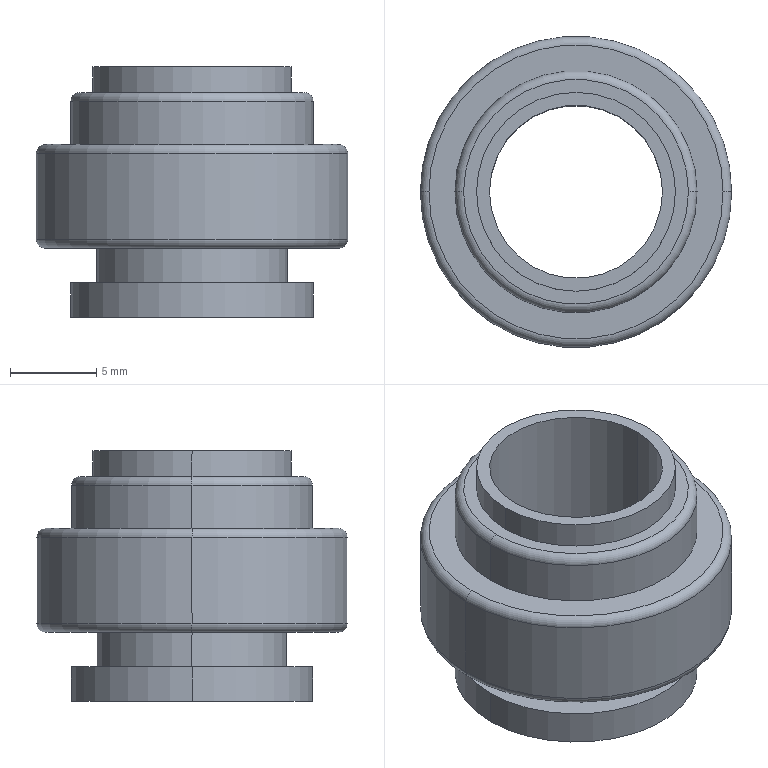Part | SolidWorks | features BaseBody 1 | 1 solid | 24 faces | box 18 x 18 x 14.5 mm | volume 1495 mm3 | cylinder 12 | plane 6 | torus 6 | commonest cylinder face diameters 14 x4 10 x2 11 x2 11.5 x2 18 x2
STEP:
#1=CARTESIAN_POINT('',(5.75,-5.,5.75));
#2=VERTEX_POINT('',#1);
#3=CARTESIAN_POINT('',(-5.75,-5.,5.75));
#4=VERTEX_POINT('',#3);
#5=CARTESIAN_POINT('',(0.,-5.,5.75));
#6=DIRECTION('',(0.,0.,1.));
#7=DIRECTION('',(1.,0.,0.));
#8=AXIS2_PLACEMENT_3D('',#5,#6,#7);
#9=CIRCLE('',#8,5.75);
#10=EDGE_CURVE('',#2,#4,#9,.T.);
#11=ORIENTED_EDGE('',*,*,#10,.F.);
#12=CARTESIAN_POINT('',(0.,-5.,5.75));
#13=DIRECTION('',(0.,0.,1.));
#14=DIRECTION('',(1.,0.,0.));
#15=AXIS2_PLACEMENT_3D('',#12,#13,#14);
#16=CIRCLE('',#15,5.75);
#17=EDGE_CURVE('',#4,#2,#16,.T.);
#18=ORIENTED_EDGE('',*,*,#17,.F.);
#19=EDGE_LOOP('',(#11,#18));
#20=FACE_BOUND('',#19,.T.);
#21=CARTESIAN_POINT('',(6.5,-5.,5.75));
#22=VERTEX_POINT('',#21);
#23=CARTESIAN_POINT('',(-6.5,-5.,5.75));
#24=VERTEX_POINT('',#23);
#25=CARTESIAN_POINT('',(0.,-5.,5.75));
#26=DIRECTION('',(0.,0.,1.));
#27=DIRECTION('',(1.,0.,0.));
#28=AXIS2_PLACEMENT_3D('',#25,#26,#27);
#29=CIRCLE('',#28,6.5);
#30=EDGE_CURVE('',#22,#24,#29,.T.);
#31=ORIENTED_EDGE('',*,*,#30,.T.);
#32=CARTESIAN_POINT('',(0.,-5.,5.75));
#33=DIRECTION('',(0.,0.,1.));
#34=DIRECTION('',(1.,0.,0.));
#35=AXIS2_PLACEMENT_3D('',#32,#33,#34);
#36=CIRCLE('',#35,6.5);
#37=EDGE_CURVE('',#24,#22,#36,.T.);
#38=ORIENTED_EDGE('',*,*,#37,.T.);
#39=EDGE_LOOP('',(#31,#38));
#40=FACE_OUTER_BOUND('',#39,.T.);
#41=CARTESIAN_POINT('',(0.,1.5,5.75));
#42=DIRECTION('',(0.,0.,-1.));
#43=DIRECTION('',(0.,-1.,0.));
#44=AXIS2_PLACEMENT_3D('',#41,#42,#43);
#45=PLANE('',#44);
#46=ADVANCED_FACE('',(#20,#40),#45,.F.);
#47=CARTESIAN_POINT('',(-5.75,-5.,7.25));
#48=VERTEX_POINT('',#47);
#49=CARTESIAN_POINT('',(-5.75,-5.,7.25));
#50=DIRECTION('',(0.,0.,1.));
#51=VECTOR('',#50,1000.);
#52=LINE('',#49,#51);
#53=EDGE_CURVE('',#4,#48,#52,.T.);
#54=ORIENTED_EDGE('',*,*,#53,.F.);
#55=ORIENTED_EDGE('',*,*,#17,.T.);
#56=CARTESIAN_POINT('',(5.75,-5.,7.25));
#57=VERTEX_POINT('',#56);
#58=CARTESIAN_POINT('',(5.75,-5.,7.25));
#59=DIRECTION('',(0.,0.,1.));
#60=VECTOR('',#59,1000.);
#61=LINE('',#58,#60);
#62=EDGE_CURVE('',#2,#57,#61,.T.);
#63=ORIENTED_EDGE('',*,*,#62,.T.);
#64=CARTESIAN_POINT('',(0.,-5.,7.25));
#65=DIRECTION('',(0.,0.,1.));
#66=DIRECTION('',(1.,0.,0.));
#67=AXIS2_PLACEMENT_3D('',#64,#65,#66);
#68=CIRCLE('',#67,5.75);
#69=EDGE_CURVE('',#48,#57,#68,.T.);
#70=ORIENTED_EDGE('',*,*,#69,.F.);
#71=EDGE_LOOP('',(#54,#55,#63,#70));
#72=FACE_OUTER_BOUND('',#71,.T.);
#73=CARTESIAN_POINT('',(0.,-5.,7.25));
#74=DIRECTION('',(0.,0.,1.));
#75=DIRECTION('',(1.,0.,0.));
#76=AXIS2_PLACEMENT_3D('',#73,#74,#75);
#77=CYLINDRICAL_SURFACE('',#76,5.75);
#78=ADVANCED_FACE('',(#72),#77,.T.);
#79=CARTESIAN_POINT('',(5.,-5.,7.25));
#80=VERTEX_POINT('',#79);
#81=CARTESIAN_POINT('',(-5.,-5.,7.25));
#82=VERTEX_POINT('',#81);
#83=CARTESIAN_POINT('',(0.,-5.,7.25));
#84=DIRECTION('',(0.,0.,1.));
#85=DIRECTION('',(1.,0.,0.));
#86=AXIS2_PLACEMENT_3D('',#83,#84,#85);
#87=CIRCLE('',#86,5.);
#88=EDGE_CURVE('',#80,#82,#87,.T.);
#89=ORIENTED_EDGE('',*,*,#88,.F.);
#90=CARTESIAN_POINT('',(0.,-5.,7.25));
#91=DIRECTION('',(0.,0.,1.));
#92=DIRECTION('',(1.,0.,0.));
#93=AXIS2_PLACEMENT_3D('',#90,#91,#92);
#94=CIRCLE('',#93,5.);
#95=EDGE_CURVE('',#82,#80,#94,.T.);
#96=ORIENTED_EDGE('',*,*,#95,.F.);
#97=EDGE_LOOP('',(#89,#96));
#98=FACE_BOUND('',#97,.T.);
#99=CARTESIAN_POINT('',(0.,-5.,7.25));
#100=DIRECTION('',(0.,0.,1.));
#101=DIRECTION('',(1.,0.,0.));
#102=AXIS2_PLACEMENT_3D('',#99,#100,#101);
#103=CIRCLE('',#102,5.75);
#104=EDGE_CURVE('',#57,#48,#103,.T.);
#105=ORIENTED_EDGE('',*,*,#104,.T.);
#106=ORIENTED_EDGE('',*,*,#69,.T.);
#107=EDGE_LOOP('',(#105,#106));
#108=FACE_OUTER_BOUND('',#107,.T.);
#109=CARTESIAN_POINT('',(0.,0.75,7.25));
#110=DIRECTION('',(0.,0.,-1.));
#111=DIRECTION('',(0.,-1.,0.));
#112=AXIS2_PLACEMENT_3D('',#109,#110,#111);
#113=PLANE('',#112);
#114=ADVANCED_FACE('',(#98,#108),#113,.F.);
#115=CARTESIAN_POINT('',(-5.,-5.,-7.25));
#116=VERTEX_POINT('',#115);
#117=CARTESIAN_POINT('',(-5.,-5.,7.25));
#118=DIRECTION('',(0.,0.,1.));
#119=VECTOR('',#118,1000.);
#120=LINE('',#117,#119);
#121=EDGE_CURVE('',#116,#82,#120,.T.);
#122=ORIENTED_EDGE('',*,*,#121,.F.);
#123=CARTESIAN_POINT('',(5.,-5.,-7.25));
#124=VERTEX_POINT('',#123);
#125=CARTESIAN_POINT('',(0.,-5.,-7.25));
#126=DIRECTION('',(0.,0.,1.));
#127=DIRECTION('',(1.,0.,0.));
#128=AXIS2_PLACEMENT_3D('',#125,#126,#127);
#129=CIRCLE('',#128,5.);
#130=EDGE_CURVE('',#124,#116,#129,.T.);
#131=ORIENTED_EDGE('',*,*,#130,.F.);
#132=CARTESIAN_POINT('',(5.,-5.,7.25));
#133=DIRECTION('',(0.,0.,1.));
#134=VECTOR('',#133,1000.);
#135=LINE('',#132,#134);
#136=EDGE_CURVE('',#124,#80,#135,.T.);
#137=ORIENTED_EDGE('',*,*,#136,.T.);
#138=ORIENTED_EDGE('',*,*,#88,.T.);
#139=EDGE_LOOP('',(#122,#131,#137,#138));
#140=FACE_OUTER_BOUND('',#139,.T.);
#141=CARTESIAN_POINT('',(0.,-5.,7.25));
#142=DIRECTION('',(0.,0.,1.));
#143=DIRECTION('',(1.,0.,0.));
#144=AXIS2_PLACEMENT_3D('',#141,#142,#143);
#145=CYLINDRICAL_SURFACE('',#144,5.);
#146=ADVANCED_FACE('',(#140),#145,.F.);
#147=ORIENTED_EDGE('',*,*,#130,.T.);
#148=CARTESIAN_POINT('',(0.,-5.,-7.25));
#149=DIRECTION('',(0.,0.,1.));
#150=DIRECTION('',(1.,0.,0.));
#151=AXIS2_PLACEMENT_3D('',#148,#149,#150);
#152=CIRCLE('',#151,5.);
#153=EDGE_CURVE('',#116,#124,#152,.T.);
#154=ORIENTED_EDGE('',*,*,#153,.T.);
#155=EDGE_LOOP('',(#147,#154));
#156=FACE_BOUND('',#155,.T.);
#157=CARTESIAN_POINT('',(7.,-5.,-7.25));
#158=VERTEX_POINT('',#157);
#159=CARTESIAN_POINT('',(-7.,-5.,-7.25));
#160=VERTEX_POINT('',#159);
#161=CARTESIAN_POINT('',(0.,-5.,-7.25));
#162=DIRECTION('',(0.,0.,1.));
#163=DIRECTION('',(1.,0.,0.));
#164=AXIS2_PLACEMENT_3D('',#161,#162,#163);
#165=CIRCLE('',#164,7.);
#166=EDGE_CURVE('',#158,#160,#165,.T.);
#167=ORIENTED_EDGE('',*,*,#166,.F.);
#168=CARTESIAN_POINT('',(0.,-5.,-7.25));
#169=DIRECTION('',(0.,0.,1.));
#170=DIRECTION('',(1.,0.,0.));
#171=AXIS2_PLACEMENT_3D('',#168,#169,#170);
#172=CIRCLE('',#171,7.);
#173=EDGE_CURVE('',#160,#158,#172,.T.);
#174=ORIENTED_EDGE('',*,*,#173,.F.);
#175=EDGE_LOOP('',(#167,#174));
#176=FACE_OUTER_BOUND('',#175,.T.);
#177=CARTESIAN_POINT('',(0.,2.,-7.25));
#178=DIRECTION('',(0.,0.,1.));
#179=DIRECTION('',(0.,-1.,0.));
#180=AXIS2_PLACEMENT_3D('',#177,#178,#179);
#181=PLANE('',#180);
#182=ADVANCED_FACE('',(#156,#176),#181,.F.);
#183=CARTESIAN_POINT('',(-7.,-5.,-5.25));
#184=VERTEX_POINT('',#183);
#185=CARTESIAN_POINT('',(-7.,-5.,7.25));
#186=DIRECTION('',(0.,0.,1.));
#187=VECTOR('',#186,1000.);
#188=LINE('',#185,#187);
#189=EDGE_CURVE('',#160,#184,#188,.T.);
#190=ORIENTED_EDGE('',*,*,#189,.F.);
#191=ORIENTED_EDGE('',*,*,#173,.T.);
#192=CARTESIAN_POINT('',(7.,-5.,-5.25));
#193=VERTEX_POINT('',#192);
#194=CARTESIAN_POINT('',(7.,-5.,7.25));
#195=DIRECTION('',(0.,0.,1.));
#196=VECTOR('',#195,1000.);
#197=LINE('',#194,#196);
#198=EDGE_CURVE('',#158,#193,#197,.T.);
#199=ORIENTED_EDGE('',*,*,#198,.T.);
#200=CARTESIAN_POINT('',(0.,-5.,-5.25));
#201=DIRECTION('',(0.,0.,1.));
#202=DIRECTION('',(1.,0.,0.));
#203=AXIS2_PLACEMENT_3D('',#200,#201,#202);
#204=CIRCLE('',#203,7.);
#205=EDGE_CURVE('',#184,#193,#204,.T.);
#206=ORIENTED_EDGE('',*,*,#205,.F.);
#207=EDGE_LOOP('',(#190,#191,#199,#206));
#208=FACE_OUTER_BOUND('',#207,.T.);
#209=CARTESIAN_POINT('',(0.,-5.,7.25));
#210=DIRECTION('',(0.,0.,1.));
#211=DIRECTION('',(1.,0.,0.));
#212=AXIS2_PLACEMENT_3D('',#209,#210,#211);
#213=CYLINDRICAL_SURFACE('',#212,7.);
#214=ADVANCED_FACE('',(#208),#213,.T.);
#215=CARTESIAN_POINT('',(5.5,-5.,-5.25));
#216=VERTEX_POINT('',#215);
#217=CARTESIAN_POINT('',(-5.5,-5.,-5.25));
#218=VERTEX_POINT('',#217);
#219=CARTESIAN_POINT('',(0.,-5.,-5.25));
#220=DIRECTION('',(0.,0.,1.));
#221=DIRECTION('',(1.,0.,0.));
#222=AXIS2_PLACEMENT_3D('',#219,#220,#221);
#223=CIRCLE('',#222,5.5);
#224=EDGE_CURVE('',#216,#218,#223,.T.);
#225=ORIENTED_EDGE('',*,*,#224,.F.);
#226=CARTESIAN_POINT('',(0.,-5.,-5.25));
#227=DIRECTION('',(0.,0.,1.));
#228=DIRECTION('',(1.,0.,0.));
#229=AXIS2_PLACEMENT_3D('',#226,#227,#228);
#230=CIRCLE('',#229,5.5);
#231=EDGE_CURVE('',#218,#216,#230,.T.);
#232=ORIENTED_EDGE('',*,*,#231,.F.);
#233=EDGE_LOOP('',(#225,#232));
#234=FACE_BOUND('',#233,.T.);
#235=CARTESIAN_POINT('',(0.,-5.,-5.25));
#236=DIRECTION('',(0.,0.,1.));
#237=DIRECTION('',(1.,0.,0.));
#238=AXIS2_PLACEMENT_3D('',#235,#236,#237);
#239=CIRCLE('',#238,7.);
#240=EDGE_CURVE('',#193,#184,#239,.T.);
#241=ORIENTED_EDGE('',*,*,#240,.T.);
#242=ORIENTED_EDGE('',*,*,#205,.T.);
#243=EDGE_LOOP('',(#241,#242));
#244=FACE_OUTER_BOUND('',#243,.T.);
#245=CARTESIAN_POINT('',(0.,2.,-5.25));
#246=DIRECTION('',(0.,0.,-1.));
#247=DIRECTION('',(0.,-1.,0.));
#248=AXIS2_PLACEMENT_3D('',#245,#246,#247);
#249=PLANE('',#248);
#250=ADVANCED_FACE('',(#234,#244),#249,.F.);
#251=CARTESIAN_POINT('',(-5.5,-5.,-3.25));
#252=VERTEX_POINT('',#251);
#253=CARTESIAN_POINT('',(-5.5,-5.,7.25));
#254=DIRECTION('',(0.,0.,1.));
#255=VECTOR('',#254,1000.);
#256=LINE('',#253,#255);
#257=EDGE_CURVE('',#218,#252,#256,.T.);
#258=ORIENTED_EDGE('',*,*,#257,.F.);
#259=ORIENTED_EDGE('',*,*,#231,.T.);
#260=CARTESIAN_POINT('',(5.5,-5.,-3.25));
#261=VERTEX_POINT('',#260);
#262=CARTESIAN_POINT('',(5.5,-5.,7.25));
#263=DIRECTION('',(0.,0.,1.));
#264=VECTOR('',#263,1000.);
#265=LINE('',#262,#264);
#266=EDGE_CURVE('',#216,#261,#265,.T.);
#267=ORIENTED_EDGE('',*,*,#266,.T.);
#268=CARTESIAN_POINT('',(0.,-5.,-3.25));
#269=DIRECTION('',(0.,0.,1.));
#270=DIRECTION('',(1.,0.,0.));
#271=AXIS2_PLACEMENT_3D('',#268,#269,#270);
#272=CIRCLE('',#271,5.5);
#273=EDGE_CURVE('',#252,#261,#272,.T.);
#274=ORIENTED_EDGE('',*,*,#273,.F.);
#275=EDGE_LOOP('',(#258,#259,#267,#274));
#276=FACE_OUTER_BOUND('',#275,.T.);
#277=CARTESIAN_POINT('',(0.,-5.,7.25));
#278=DIRECTION('',(0.,0.,1.));
#279=DIRECTION('',(1.,0.,0.));
#280=AXIS2_PLACEMENT_3D('',#277,#278,#279);
#281=CYLINDRICAL_SURFACE('',#280,5.5);
#282=ADVANCED_FACE('',(#276),#281,.T.);
#283=CARTESIAN_POINT('',(0.,-5.,-3.25));
#284=DIRECTION('',(0.,0.,1.));
#285=DIRECTION('',(1.,0.,0.));
#286=AXIS2_PLACEMENT_3D('',#283,#284,#285);
#287=CIRCLE('',#286,5.5);
#288=EDGE_CURVE('',#261,#252,#287,.T.);
#289=ORIENTED_EDGE('',*,*,#288,.T.);
#290=ORIENTED_EDGE('',*,*,#273,.T.);
#291=EDGE_LOOP('',(#289,#290));
#292=FACE_BOUND('',#291,.T.);
#293=CARTESIAN_POINT('',(8.5,-5.,-3.25));
#294=VERTEX_POINT('',#293);
#295=CARTESIAN_POINT('',(-8.5,-5.,-3.25));
#296=VERTEX_POINT('',#295);
#297=CARTESIAN_POINT('',(0.,-5.,-3.25));
#298=DIRECTION('',(0.,0.,1.));
#299=DIRECTION('',(1.,0.,0.));
#300=AXIS2_PLACEMENT_3D('',#297,#298,#299);
#301=CIRCLE('',#300,8.5);
#302=EDGE_CURVE('',#294,#296,#301,.T.);
#303=ORIENTED_EDGE('',*,*,#302,.F.);
#304=CARTESIAN_POINT('',(0.,-5.,-3.25));
#305=DIRECTION('',(0.,0.,1.));
#306=DIRECTION('',(1.,0.,0.));
#307=AXIS2_PLACEMENT_3D('',#304,#305,#306);
#308=CIRCLE('',#307,8.5);
#309=EDGE_CURVE('',#296,#294,#308,.T.);
#310=ORIENTED_EDGE('',*,*,#309,.F.);
#311=EDGE_LOOP('',(#303,#310));
#312=FACE_OUTER_BOUND('',#311,.T.);
#313=CARTESIAN_POINT('',(0.,0.5,-3.25));
#314=DIRECTION('',(0.,0.,1.));
#315=DIRECTION('',(0.,-1.,0.));
#316=AXIS2_PLACEMENT_3D('',#313,#314,#315);
#317=PLANE('',#316);
#318=ADVANCED_FACE('',(#292,#312),#317,.F.);
#319=CARTESIAN_POINT('',(-9.,-5.,-2.75));
#320=VERTEX_POINT('',#319);
#321=CARTESIAN_POINT('',(-8.5,-5.,-2.75));
#322=DIRECTION('',(0.,1.,0.));
#323=DIRECTION('',(-1.,0.,0.));
#324=AXIS2_PLACEMENT_3D('',#321,#322,#323);
#325=CIRCLE('',#324,0.5);
#326=EDGE_CURVE('',#296,#320,#325,.T.);
#327=ORIENTED_EDGE('',*,*,#326,.F.);
#328=ORIENTED_EDGE('',*,*,#309,.T.);
#329=CARTESIAN_POINT('',(9.,-5.,-2.75));
#330=VERTEX_POINT('',#329);
#331=CARTESIAN_POINT('',(8.5,-5.,-2.75));
#332=DIRECTION('',(0.,-1.,0.));
#333=DIRECTION('',(0.,0.,-1.));
#334=AXIS2_PLACEMENT_3D('',#331,#332,#333);
#335=CIRCLE('',#334,0.5);
#336=EDGE_CURVE('',#294,#330,#335,.T.);
#337=ORIENTED_EDGE('',*,*,#336,.T.);
#338=CARTESIAN_POINT('',(0.,-5.,-2.75));
#339=DIRECTION('',(0.,0.,1.));
#340=DIRECTION('',(1.,0.,0.));
#341=AXIS2_PLACEMENT_3D('',#338,#339,#340);
#342=CIRCLE('',#341,9.);
#343=EDGE_CURVE('',#320,#330,#342,.T.);
#344=ORIENTED_EDGE('',*,*,#343,.F.);
#345=EDGE_LOOP('',(#327,#328,#337,#344));
#346=FACE_OUTER_BOUND('',#345,.T.);
#347=CARTESIAN_POINT('',(0.,-5.,-2.75));
#348=DIRECTION('',(0.,0.,1.));
#349=DIRECTION('',(1.,0.,0.));
#350=AXIS2_PLACEMENT_3D('',#347,#348,#349);
#351=TOROIDAL_SURFACE('',#350,8.5,0.5);
#352=ADVANCED_FACE('',(#346),#351,.T.);
#353=CARTESIAN_POINT('',(-9.,-5.,2.25));
#354=VERTEX_POINT('',#353);
#355=CARTESIAN_POINT('',(-9.,-5.,7.25));
#356=DIRECTION('',(0.,0.,1.));
#357=VECTOR('',#356,1000.);
#358=LINE('',#355,#357);
#359=EDGE_CURVE('',#320,#354,#358,.T.);
#360=ORIENTED_EDGE('',*,*,#359,.F.);
#361=ORIENTED_EDGE('',*,*,#343,.T.);
#362=CARTESIAN_POINT('',(9.,-5.,2.25));
#363=VERTEX_POINT('',#362);
#364=CARTESIAN_POINT('',(9.,-5.,7.25));
#365=DIRECTION('',(0.,0.,1.));
#366=VECTOR('',#365,1000.);
#367=LINE('',#364,#366);
#368=EDGE_CURVE('',#330,#363,#367,.T.);
#369=ORIENTED_EDGE('',*,*,#368,.T.);
#370=CARTESIAN_POINT('',(0.,-5.,2.25));
#371=DIRECTION('',(0.,0.,1.));
#372=DIRECTION('',(1.,0.,0.));
#373=AXIS2_PLACEMENT_3D('',#370,#371,#372);
#374=CIRCLE('',#373,9.);
#375=EDGE_CURVE('',#354,#363,#374,.T.);
#376=ORIENTED_EDGE('',*,*,#375,.F.);
#377=EDGE_LOOP('',(#360,#361,#369,#376));
#378=FACE_OUTER_BOUND('',#377,.T.);
#379=CARTESIAN_POINT('',(0.,-5.,7.25));
#380=DIRECTION('',(0.,0.,1.));
#381=DIRECTION('',(1.,0.,0.));
#382=AXIS2_PLACEMENT_3D('',#379,#380,#381);
#383=CYLINDRICAL_SURFACE('',#382,9.);
#384=ADVANCED_FACE('',(#378),#383,.T.);
#385=CARTESIAN_POINT('',(-8.5,-5.,2.75));
#386=VERTEX_POINT('',#385);
#387=CARTESIAN_POINT('',(-8.5,-5.,2.25));
#388=DIRECTION('',(0.,1.,0.));
#389=DIRECTION('',(-1.,0.,0.));
#390=AXIS2_PLACEMENT_3D('',#387,#388,#389);
#391=CIRCLE('',#390,0.5);
#392=EDGE_CURVE('',#354,#386,#391,.T.);
#393=ORIENTED_EDGE('',*,*,#392,.F.);
#394=ORIENTED_EDGE('',*,*,#375,.T.);
#395=CARTESIAN_POINT('',(8.5,-5.,2.75));
#396=VERTEX_POINT('',#395);
#397=CARTESIAN_POINT('',(8.5,-5.,2.25));
#398=DIRECTION('',(0.,-1.,0.));
#399=DIRECTION('',(0.,0.,-1.));
#400=AXIS2_PLACEMENT_3D('',#397,#398,#399);
#401=CIRCLE('',#400,0.5);
#402=EDGE_CURVE('',#363,#396,#401,.T.);
#403=ORIENTED_EDGE('',*,*,#402,.T.);
#404=CARTESIAN_POINT('',(0.,-5.,2.75));
#405=DIRECTION('',(0.,0.,1.));
#406=DIRECTION('',(1.,0.,0.));
#407=AXIS2_PLACEMENT_3D('',#404,#405,#406);
#408=CIRCLE('',#407,8.5);
#409=EDGE_CURVE('',#386,#396,#408,.T.);
#410=ORIENTED_EDGE('',*,*,#409,.F.);
#411=EDGE_LOOP('',(#393,#394,#403,#410));
#412=FACE_OUTER_BOUND('',#411,.T.);
#413=CARTESIAN_POINT('',(0.,-5.,2.25));
#414=DIRECTION('',(0.,0.,1.));
#415=DIRECTION('',(1.,0.,0.));
#416=AXIS2_PLACEMENT_3D('',#413,#414,#415);
#417=TOROIDAL_SURFACE('',#416,8.5,0.5);
#418=ADVANCED_FACE('',(#412),#417,.T.);
#419=CARTESIAN_POINT('',(7.,-5.,2.75));
#420=VERTEX_POINT('',#419);
#421=CARTESIAN_POINT('',(-7.,-5.,2.75));
#422=VERTEX_POINT('',#421);
#423=CARTESIAN_POINT('',(0.,-5.,2.75));
#424=DIRECTION('',(0.,0.,1.));
#425=DIRECTION('',(1.,0.,0.));
#426=AXIS2_PLACEMENT_3D('',#423,#424,#425);
#427=CIRCLE('',#426,7.);
#428=EDGE_CURVE('',#420,#422,#427,.T.);
#429=ORIENTED_EDGE('',*,*,#428,.F.);
#430=CARTESIAN_POINT('',(0.,-5.,2.75));
#431=DIRECTION('',(0.,0.,1.));
#432=DIRECTION('',(1.,0.,0.));
#433=AXIS2_PLACEMENT_3D('',#430,#431,#432);
#434=CIRCLE('',#433,7.);
#435=EDGE_CURVE('',#422,#420,#434,.T.);
#436=ORIENTED_EDGE('',*,*,#435,.F.);
#437=EDGE_LOOP('',(#429,#436));
#438=FACE_BOUND('',#437,.T.);
#439=CARTESIAN_POINT('',(0.,-5.,2.75));
#440=DIRECTION('',(0.,0.,1.));
#441=DIRECTION('',(1.,0.,0.));
#442=AXIS2_PLACEMENT_3D('',#439,#440,#441);
#443=CIRCLE('',#442,8.5);
#444=EDGE_CURVE('',#396,#386,#443,.T.);
#445=ORIENTED_EDGE('',*,*,#444,.T.);
#446=ORIENTED_EDGE('',*,*,#409,.T.);
#447=EDGE_LOOP('',(#445,#446));
#448=FACE_OUTER_BOUND('',#447,.T.);
#449=CARTESIAN_POINT('',(0.,3.5,2.75));
#450=DIRECTION('',(0.,0.,-1.));
#451=DIRECTION('',(0.,-1.,0.));
#452=AXIS2_PLACEMENT_3D('',#449,#450,#451);
#453=PLANE('',#452);
#454=ADVANCED_FACE('',(#438,#448),#453,.F.);
#455=CARTESIAN_POINT('',(-7.,-5.,5.25));
#456=VERTEX_POINT('',#455);
#457=CARTESIAN_POINT('',(-7.,-5.,7.25));
#458=DIRECTION('',(0.,0.,1.));
#459=VECTOR('',#458,1000.);
#460=LINE('',#457,#459);
#461=EDGE_CURVE('',#422,#456,#460,.T.);
#462=ORIENTED_EDGE('',*,*,#461,.F.);
#463=ORIENTED_EDGE('',*,*,#435,.T.);
#464=CARTESIAN_POINT('',(7.,-5.,5.25));
#465=VERTEX_POINT('',#464);
#466=CARTESIAN_POINT('',(7.,-5.,7.25));
#467=DIRECTION('',(0.,0.,1.));
#468=VECTOR('',#467,1000.);
#469=LINE('',#466,#468);
#470=EDGE_CURVE('',#420,#465,#469,.T.);
#471=ORIENTED_EDGE('',*,*,#470,.T.);
#472=CARTESIAN_POINT('',(0.,-5.,5.25));
#473=DIRECTION('',(0.,0.,1.));
#474=DIRECTION('',(1.,0.,0.));
#475=AXIS2_PLACEMENT_3D('',#472,#473,#474);
#476=CIRCLE('',#475,7.);
#477=EDGE_CURVE('',#456,#465,#476,.T.);
#478=ORIENTED_EDGE('',*,*,#477,.F.);
#479=EDGE_LOOP('',(#462,#463,#471,#478));
#480=FACE_OUTER_BOUND('',#479,.T.);
#481=CARTESIAN_POINT('',(0.,-5.,7.25));
#482=DIRECTION('',(0.,0.,1.));
#483=DIRECTION('',(1.,0.,0.));
#484=AXIS2_PLACEMENT_3D('',#481,#482,#483);
#485=CYLINDRICAL_SURFACE('',#484,7.);
#486=ADVANCED_FACE('',(#480),#485,.T.);
#487=CARTESIAN_POINT('',(-6.5,-5.,5.25));
#488=DIRECTION('',(0.,1.,0.));
#489=DIRECTION('',(-1.,0.,0.));
#490=AXIS2_PLACEMENT_3D('',#487,#488,#489);
#491=CIRCLE('',#490,0.5);
#492=EDGE_CURVE('',#456,#24,#491,.T.);
#493=ORIENTED_EDGE('',*,*,#492,.F.);
#494=ORIENTED_EDGE('',*,*,#477,.T.);
#495=CARTESIAN_POINT('',(6.5,-5.,5.25));
#496=DIRECTION('',(0.,-1.,0.));
#497=DIRECTION('',(0.,0.,-1.));
#498=AXIS2_PLACEMENT_3D('',#495,#496,#497);
#499=CIRCLE('',#498,0.5);
#500=EDGE_CURVE('',#465,#22,#499,.T.);
#501=ORIENTED_EDGE('',*,*,#500,.T.);
#502=ORIENTED_EDGE('',*,*,#37,.F.);
#503=EDGE_LOOP('',(#493,#494,#501,#502));
#504=FACE_OUTER_BOUND('',#503,.T.);
#505=CARTESIAN_POINT('',(0.,-5.,5.25));
#506=DIRECTION('',(0.,0.,1.));
#507=DIRECTION('',(1.,0.,0.));
#508=AXIS2_PLACEMENT_3D('',#505,#506,#507);
#509=TOROIDAL_SURFACE('',#508,6.5,0.5);
#510=ADVANCED_FACE('',(#504),#509,.T.);
#511=CARTESIAN_POINT('',(0.,-5.,5.25));
#512=DIRECTION('',(0.,0.,1.));
#513=DIRECTION('',(1.,0.,0.));
#514=AXIS2_PLACEMENT_3D('',#511,#512,#513);
#515=CIRCLE('',#514,7.);
#516=EDGE_CURVE('',#465,#456,#515,.T.);
#517=ORIENTED_EDGE('',*,*,#516,.T.);
#518=ORIENTED_EDGE('',*,*,#492,.T.);
#519=ORIENTED_EDGE('',*,*,#30,.F.);
#520=ORIENTED_EDGE('',*,*,#500,.F.);
#521=EDGE_LOOP('',(#517,#518,#519,#520));
#522=FACE_OUTER_BOUND('',#521,.T.);
#523=CARTESIAN_POINT('',(0.,-5.,5.25));
#524=DIRECTION('',(0.,0.,1.));
#525=DIRECTION('',(1.,0.,0.));
#526=AXIS2_PLACEMENT_3D('',#523,#524,#525);
#527=TOROIDAL_SURFACE('',#526,6.5,0.5);
#528=ADVANCED_FACE('',(#522),#527,.T.);
#529=ORIENTED_EDGE('',*,*,#428,.T.);
#530=ORIENTED_EDGE('',*,*,#461,.T.);
#531=ORIENTED_EDGE('',*,*,#516,.F.);
#532=ORIENTED_EDGE('',*,*,#470,.F.);
#533=EDGE_LOOP('',(#529,#530,#531,#532));
#534=FACE_OUTER_BOUND('',#533,.T.);
#535=CARTESIAN_POINT('',(0.,-5.,7.25));
#536=DIRECTION('',(0.,0.,1.));
#537=DIRECTION('',(1.,0.,0.));
#538=AXIS2_PLACEMENT_3D('',#535,#536,#537);
#539=CYLINDRICAL_SURFACE('',#538,7.);
#540=ADVANCED_FACE('',(#534),#539,.T.);
#541=CARTESIAN_POINT('',(0.,-5.,2.25));
#542=DIRECTION('',(0.,0.,1.));
#543=DIRECTION('',(1.,0.,0.));
#544=AXIS2_PLACEMENT_3D('',#541,#542,#543);
#545=CIRCLE('',#544,9.);
#546=EDGE_CURVE('',#363,#354,#545,.T.);
#547=ORIENTED_EDGE('',*,*,#546,.T.);
#548=ORIENTED_EDGE('',*,*,#392,.T.);
#549=ORIENTED_EDGE('',*,*,#444,.F.);
#550=ORIENTED_EDGE('',*,*,#402,.F.);
#551=EDGE_LOOP('',(#547,#548,#549,#550));
#552=FACE_OUTER_BOUND('',#551,.T.);
#553=CARTESIAN_POINT('',(0.,-5.,2.25));
#554=DIRECTION('',(0.,0.,1.));
#555=DIRECTION('',(1.,0.,0.));
#556=AXIS2_PLACEMENT_3D('',#553,#554,#555);
#557=TOROIDAL_SURFACE('',#556,8.5,0.5);
#558=ADVANCED_FACE('',(#552),#557,.T.);
#559=CARTESIAN_POINT('',(0.,-5.,-2.75));
#560=DIRECTION('',(0.,0.,1.));
#561=DIRECTION('',(1.,0.,0.));
#562=AXIS2_PLACEMENT_3D('',#559,#560,#561);
#563=CIRCLE('',#562,9.);
#564=EDGE_CURVE('',#330,#320,#563,.T.);
#565=ORIENTED_EDGE('',*,*,#564,.T.);
#566=ORIENTED_EDGE('',*,*,#359,.T.);
#567=ORIENTED_EDGE('',*,*,#546,.F.);
#568=ORIENTED_EDGE('',*,*,#368,.F.);
#569=EDGE_LOOP('',(#565,#566,#567,#568));
#570=FACE_OUTER_BOUND('',#569,.T.);
#571=CARTESIAN_POINT('',(0.,-5.,7.25));
#572=DIRECTION('',(0.,0.,1.));
#573=DIRECTION('',(1.,0.,0.));
#574=AXIS2_PLACEMENT_3D('',#571,#572,#573);
#575=CYLINDRICAL_SURFACE('',#574,9.);
#576=ADVANCED_FACE('',(#570),#575,.T.);
#577=ORIENTED_EDGE('',*,*,#302,.T.);
#578=ORIENTED_EDGE('',*,*,#326,.T.);
#579=ORIENTED_EDGE('',*,*,#564,.F.);
#580=ORIENTED_EDGE('',*,*,#336,.F.);
#581=EDGE_LOOP('',(#577,#578,#579,#580));
#582=FACE_OUTER_BOUND('',#581,.T.);
#583=CARTESIAN_POINT('',(0.,-5.,-2.75));
#584=DIRECTION('',(0.,0.,1.));
#585=DIRECTION('',(1.,0.,0.));
#586=AXIS2_PLACEMENT_3D('',#583,#584,#585);
#587=TOROIDAL_SURFACE('',#586,8.5,0.5);
#588=ADVANCED_FACE('',(#582),#587,.T.);
#589=ORIENTED_EDGE('',*,*,#224,.T.);
#590=ORIENTED_EDGE('',*,*,#257,.T.);
#591=ORIENTED_EDGE('',*,*,#288,.F.);
#592=ORIENTED_EDGE('',*,*,#266,.F.);
#593=EDGE_LOOP('',(#589,#590,#591,#592));
#594=FACE_OUTER_BOUND('',#593,.T.);
#595=CARTESIAN_POINT('',(0.,-5.,7.25));
#596=DIRECTION('',(0.,0.,1.));
#597=DIRECTION('',(1.,0.,0.));
#598=AXIS2_PLACEMENT_3D('',#595,#596,#597);
#599=CYLINDRICAL_SURFACE('',#598,5.5);
#600=ADVANCED_FACE('',(#594),#599,.T.);
#601=ORIENTED_EDGE('',*,*,#166,.T.);
#602=ORIENTED_EDGE('',*,*,#189,.T.);
#603=ORIENTED_EDGE('',*,*,#240,.F.);
#604=ORIENTED_EDGE('',*,*,#198,.F.);
#605=EDGE_LOOP('',(#601,#602,#603,#604));
#606=FACE_OUTER_BOUND('',#605,.T.);
#607=CARTESIAN_POINT('',(0.,-5.,7.25));
#608=DIRECTION('',(0.,0.,1.));
#609=DIRECTION('',(1.,0.,0.));
#610=AXIS2_PLACEMENT_3D('',#607,#608,#609);
#611=CYLINDRICAL_SURFACE('',#610,7.);
#612=ADVANCED_FACE('',(#606),#611,.T.);
#613=ORIENTED_EDGE('',*,*,#153,.F.);
#614=ORIENTED_EDGE('',*,*,#121,.T.);
#615=ORIENTED_EDGE('',*,*,#95,.T.);
#616=ORIENTED_EDGE('',*,*,#136,.F.);
#617=EDGE_LOOP('',(#613,#614,#615,#616));
#618=FACE_OUTER_BOUND('',#617,.T.);
#619=CARTESIAN_POINT('',(0.,-5.,7.25));
#620=DIRECTION('',(0.,0.,1.));
#621=DIRECTION('',(1.,0.,0.));
#622=AXIS2_PLACEMENT_3D('',#619,#620,#621);
#623=CYLINDRICAL_SURFACE('',#622,5.);
#624=ADVANCED_FACE('',(#618),#623,.F.);
#625=ORIENTED_EDGE('',*,*,#10,.T.);
#626=ORIENTED_EDGE('',*,*,#53,.T.);
#627=ORIENTED_EDGE('',*,*,#104,.F.);
#628=ORIENTED_EDGE('',*,*,#62,.F.);
#629=EDGE_LOOP('',(#625,#626,#627,#628));
#630=FACE_OUTER_BOUND('',#629,.T.);
#631=CARTESIAN_POINT('',(0.,-5.,7.25));
#632=DIRECTION('',(0.,0.,1.));
#633=DIRECTION('',(1.,0.,0.));
#634=AXIS2_PLACEMENT_3D('',#631,#632,#633);
#635=CYLINDRICAL_SURFACE('',#634,5.75);
#636=ADVANCED_FACE('',(#630),#635,.T.);
#637=CLOSED_SHELL('',(#46,#78,#114,#146,#182,#214,#250,#282,#318,#352,#384,#418,#454,#486,#510,#528,#540,#558,#576,#588,#600,#612,#624,#636));
#638=MANIFOLD_SOLID_BREP('',#637);
#639=CARTESIAN_POINT('',(0.,0.,0.));
#640=DIRECTION('',(0.,0.,1.));
#641=DIRECTION('',(1.,0.,0.));
#642=AXIS2_PLACEMENT_3D('',#639,#640,#641);
#643=(LENGTH_UNIT()NAMED_UNIT(*)SI_UNIT(.MILLI.,.METRE.));
#644=UNCERTAINTY_MEASURE_WITH_UNIT(LENGTH_MEASURE(0.00001),#643,'','');
#645=(NAMED_UNIT(*)PLANE_ANGLE_UNIT()SI_UNIT($,.RADIAN.));
#646=(NAMED_UNIT(*)SI_UNIT($,.STERADIAN.)SOLID_ANGLE_UNIT());
#647=(GEOMETRIC_REPRESENTATION_CONTEXT(3)GLOBAL_UNCERTAINTY_ASSIGNED_CONTEXT((#644))GLOBAL_UNIT_ASSIGNED_CONTEXT((#643,#645,#646))REPRESENTATION_CONTEXT('',''));
#648=ADVANCED_BREP_SHAPE_REPRESENTATION('',(#638,#642),#647);